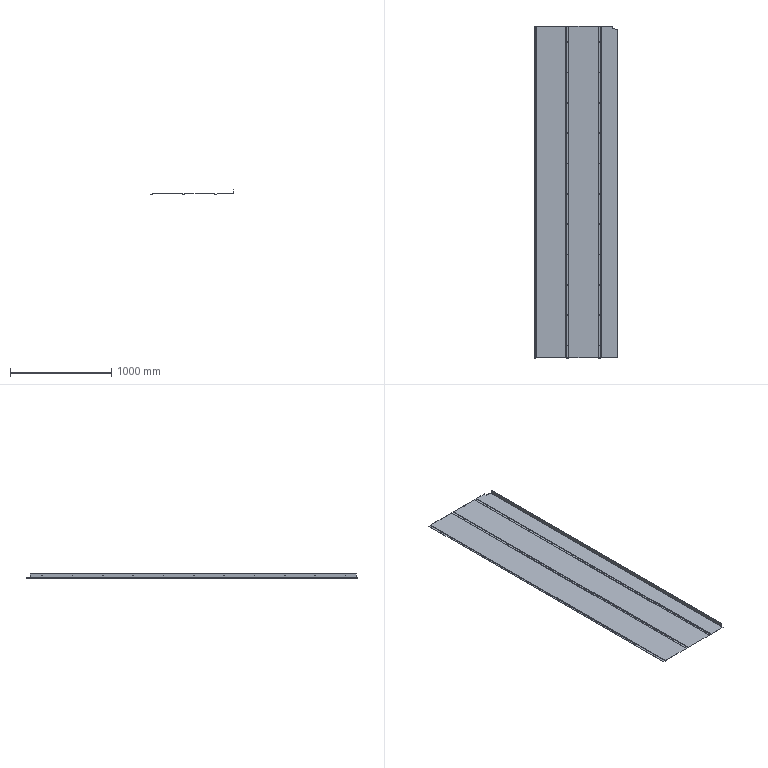Part | STEP file | TS-S99 | 1 solid | 191 faces | box 830 x 3283 x 43 mm | volume 3438699 mm3 | cylinder 113 | plane 78 | commonest cylinder face diameters 5.4 x88 0.4 x11 2.8 x11 10 x1 14 x1 16 x1